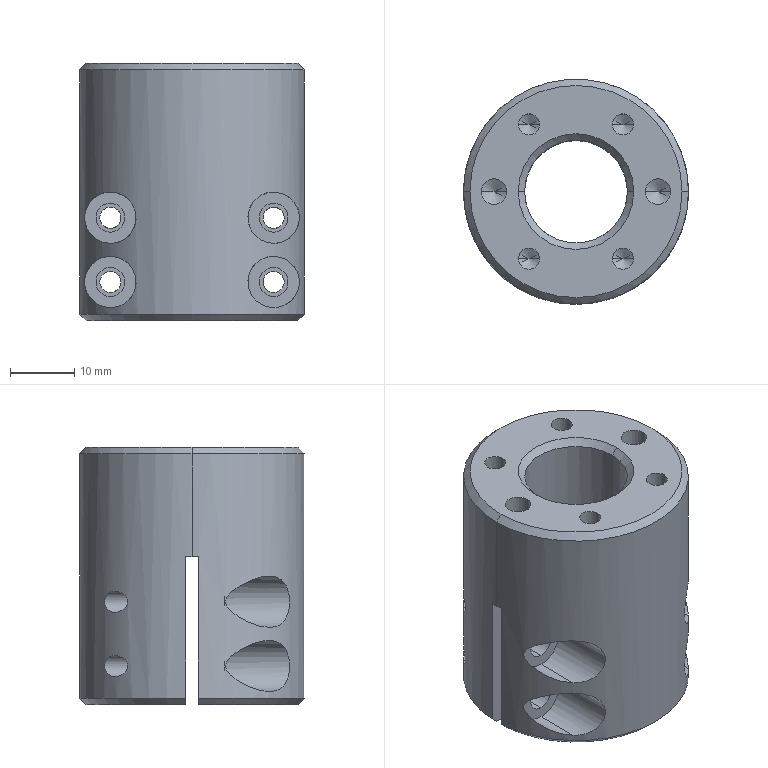Part | STEP file | 11-FG-SB01011 | 1 solid | 73 faces | box 35 x 35 x 40 mm | volume 26701 mm3 | cylinder 40 | cone 20 | plane 13 | commonest cylinder face diameters 3.3 x16 4.5 x8 8 x8 4 x4 16 x2 35 x2